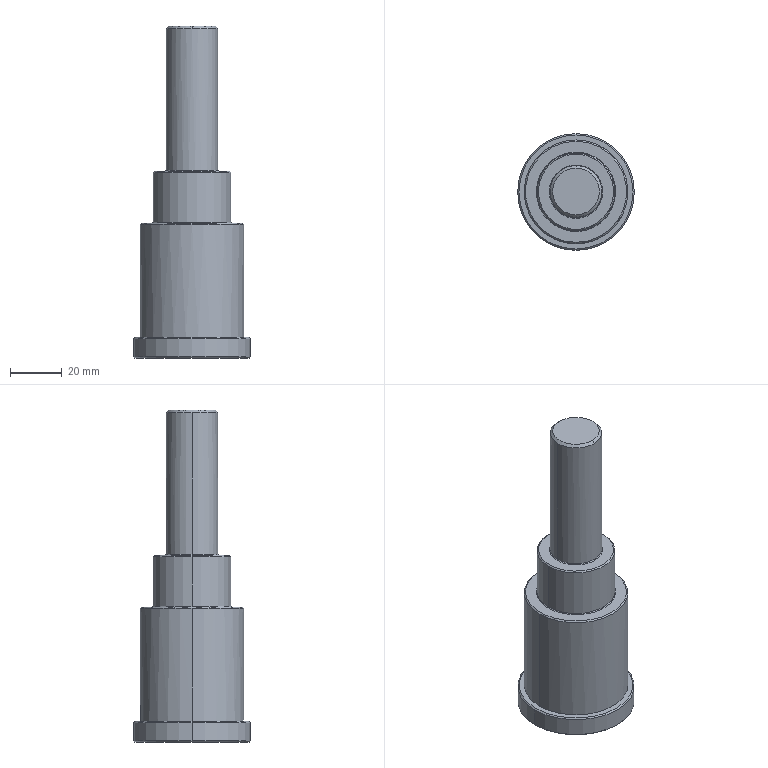Part | STEP file | 1 solid | 27 faces | box 45 x 45 x 128 mm | volume 99657 mm3 | cone 10 | cylinder 8 | plane 5 | spline 4 | commonest cylinder face diameters 20 x2 30 x2 40 x2 45 x2